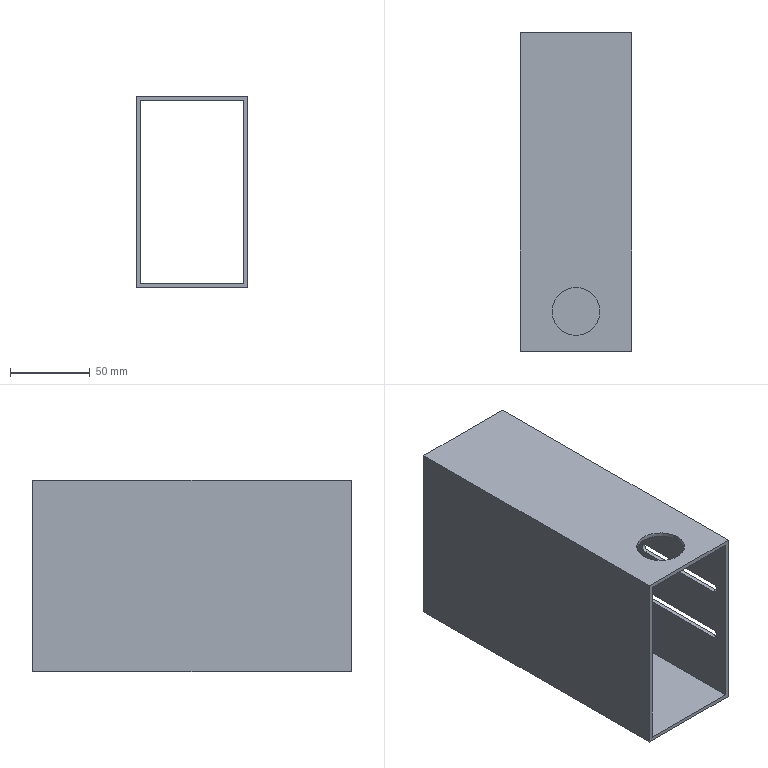Part | SolidWorks | features HoleWzd 2, Cut 1, Extrusion 1, ICE 1 | 1 solid | 34 faces | box 70 x 200 x 120 mm | volume 169957 mm3 | plane 22 | cylinder 12 | commonest cylinder face diameters 4.8 x6 5.8 x4 30 x2
STEP:
#1=CARTESIAN_POINT('',(67.5,52.4,-68.5));
#2=VERTEX_POINT('',#1);
#3=CARTESIAN_POINT('',(67.5,50.,-70.9));
#4=VERTEX_POINT('',#3);
#5=CARTESIAN_POINT('',(67.5,50.,-68.5));
#6=DIRECTION('',(-1.,0.,0.));
#7=DIRECTION('',(0.,0.,1.));
#8=AXIS2_PLACEMENT_3D('',#5,#6,#7);
#9=CIRCLE('',#8,2.4);
#10=EDGE_CURVE('',#2,#4,#9,.T.);
#11=ORIENTED_EDGE('',*,*,#10,.T.);
#12=CARTESIAN_POINT('',(70.,50.,-70.9));
#13=VERTEX_POINT('',#12);
#14=CARTESIAN_POINT('',(70.,50.,-70.9));
#15=DIRECTION('',(1.,0.,0.));
#16=VECTOR('',#15,1000.);
#17=LINE('',#14,#16);
#18=EDGE_CURVE('',#4,#13,#17,.T.);
#19=ORIENTED_EDGE('',*,*,#18,.T.);
#20=CARTESIAN_POINT('',(70.,52.4,-68.5));
#21=VERTEX_POINT('',#20);
#22=CARTESIAN_POINT('',(70.,50.,-68.5));
#23=DIRECTION('',(1.,0.,0.));
#24=DIRECTION('',(0.,0.,-1.));
#25=AXIS2_PLACEMENT_3D('',#22,#23,#24);
#26=CIRCLE('',#25,2.4);
#27=EDGE_CURVE('',#13,#21,#26,.T.);
#28=ORIENTED_EDGE('',*,*,#27,.T.);
#29=CARTESIAN_POINT('',(67.499,52.4,-68.5));
#30=DIRECTION('',(-1.,0.,0.));
#31=VECTOR('',#30,1000.);
#32=LINE('',#29,#31);
#33=EDGE_CURVE('',#21,#2,#32,.T.);
#34=ORIENTED_EDGE('',*,*,#33,.T.);
#35=EDGE_LOOP('',(#11,#19,#28,#34));
#36=FACE_OUTER_BOUND('',#35,.T.);
#37=CARTESIAN_POINT('',(70.,50.,-68.5));
#38=DIRECTION('',(1.,0.,0.));
#39=DIRECTION('',(0.,0.,-1.));
#40=AXIS2_PLACEMENT_3D('',#37,#38,#39);
#41=CYLINDRICAL_SURFACE('',#40,2.4);
#42=ADVANCED_FACE('',(#36),#41,.F.);
#43=CARTESIAN_POINT('',(67.5,22.4,-68.5));
#44=VERTEX_POINT('',#43);
#45=CARTESIAN_POINT('',(67.5,20.,-70.9));
#46=VERTEX_POINT('',#45);
#47=CARTESIAN_POINT('',(67.5,20.,-68.5));
#48=DIRECTION('',(-1.,0.,0.));
#49=DIRECTION('',(0.,0.,1.));
#50=AXIS2_PLACEMENT_3D('',#47,#48,#49);
#51=CIRCLE('',#50,2.4);
#52=EDGE_CURVE('',#44,#46,#51,.T.);
#53=ORIENTED_EDGE('',*,*,#52,.T.);
#54=CARTESIAN_POINT('',(70.,20.,-70.9));
#55=VERTEX_POINT('',#54);
#56=CARTESIAN_POINT('',(70.,20.,-70.9));
#57=DIRECTION('',(1.,0.,0.));
#58=VECTOR('',#57,1000.);
#59=LINE('',#56,#58);
#60=EDGE_CURVE('',#46,#55,#59,.T.);
#61=ORIENTED_EDGE('',*,*,#60,.T.);
#62=CARTESIAN_POINT('',(70.,22.4,-68.5));
#63=VERTEX_POINT('',#62);
#64=CARTESIAN_POINT('',(70.,20.,-68.5));
#65=DIRECTION('',(1.,0.,0.));
#66=DIRECTION('',(0.,0.,-1.));
#67=AXIS2_PLACEMENT_3D('',#64,#65,#66);
#68=CIRCLE('',#67,2.4);
#69=EDGE_CURVE('',#55,#63,#68,.T.);
#70=ORIENTED_EDGE('',*,*,#69,.T.);
#71=CARTESIAN_POINT('',(67.499,22.4,-68.5));
#72=DIRECTION('',(-1.,0.,0.));
#73=VECTOR('',#72,1000.);
#74=LINE('',#71,#73);
#75=EDGE_CURVE('',#63,#44,#74,.T.);
#76=ORIENTED_EDGE('',*,*,#75,.T.);
#77=EDGE_LOOP('',(#53,#61,#70,#76));
#78=FACE_OUTER_BOUND('',#77,.T.);
#79=CARTESIAN_POINT('',(70.,20.,-68.5));
#80=DIRECTION('',(1.,0.,0.));
#81=DIRECTION('',(0.,0.,-1.));
#82=AXIS2_PLACEMENT_3D('',#79,#80,#81);
#83=CYLINDRICAL_SURFACE('',#82,2.4);
#84=ADVANCED_FACE('',(#78),#83,.F.);
#85=CARTESIAN_POINT('',(20.,-75.,-2.5));
#86=VERTEX_POINT('',#85);
#87=CARTESIAN_POINT('',(50.,-75.,-2.5));
#88=VERTEX_POINT('',#87);
#89=CARTESIAN_POINT('',(35.,-75.,-2.5));
#90=DIRECTION('',(0.,0.,1.));
#91=DIRECTION('',(-1.,0.,0.));
#92=AXIS2_PLACEMENT_3D('',#89,#90,#91);
#93=CIRCLE('',#92,15.);
#94=EDGE_CURVE('',#86,#88,#93,.T.);
#95=ORIENTED_EDGE('',*,*,#94,.F.);
#96=CARTESIAN_POINT('',(20.,-75.,0.));
#97=VERTEX_POINT('',#96);
#98=CARTESIAN_POINT('',(20.,-75.,-120.001));
#99=DIRECTION('',(0.,0.,1.));
#100=VECTOR('',#99,1000.);
#101=LINE('',#98,#100);
#102=EDGE_CURVE('',#86,#97,#101,.T.);
#103=ORIENTED_EDGE('',*,*,#102,.T.);
#104=CARTESIAN_POINT('',(50.,-75.,0.));
#105=VERTEX_POINT('',#104);
#106=CARTESIAN_POINT('',(35.,-75.,0.));
#107=DIRECTION('',(0.,0.,1.));
#108=DIRECTION('',(1.,0.,0.));
#109=AXIS2_PLACEMENT_3D('',#106,#107,#108);
#110=CIRCLE('',#109,15.);
#111=EDGE_CURVE('',#97,#105,#110,.T.);
#112=ORIENTED_EDGE('',*,*,#111,.T.);
#113=CARTESIAN_POINT('',(50.,-75.,-120.001));
#114=DIRECTION('',(0.,0.,1.));
#115=VECTOR('',#114,1000.);
#116=LINE('',#113,#115);
#117=EDGE_CURVE('',#88,#105,#116,.T.);
#118=ORIENTED_EDGE('',*,*,#117,.F.);
#119=EDGE_LOOP('',(#95,#103,#112,#118));
#120=FACE_OUTER_BOUND('',#119,.T.);
#121=CARTESIAN_POINT('',(35.,-75.,-120.001));
#122=DIRECTION('',(0.,0.,1.));
#123=DIRECTION('',(1.,0.,0.));
#124=AXIS2_PLACEMENT_3D('',#121,#122,#123);
#125=CYLINDRICAL_SURFACE('',#124,15.);
#126=ADVANCED_FACE('',(#120),#125,.F.);
#127=CARTESIAN_POINT('',(70.,-89.,-43.452));
#128=VERTEX_POINT('',#127);
#129=CARTESIAN_POINT('',(70.,-29.,-43.452));
#130=VERTEX_POINT('',#129);
#131=CARTESIAN_POINT('',(70.,-89.,-43.452));
#132=DIRECTION('',(0.,1.,0.));
#133=VECTOR('',#132,1000.);
#134=LINE('',#131,#133);
#135=EDGE_CURVE('',#128,#130,#134,.T.);
#136=ORIENTED_EDGE('',*,*,#135,.F.);
#137=CARTESIAN_POINT('',(70.,-89.,-37.652));
#138=VERTEX_POINT('',#137);
#139=CARTESIAN_POINT('',(70.,-89.,-40.552));
#140=DIRECTION('',(1.,0.,0.));
#141=DIRECTION('',(0.,0.,-1.));
#142=AXIS2_PLACEMENT_3D('',#139,#140,#141);
#143=CIRCLE('',#142,2.9);
#144=EDGE_CURVE('',#138,#128,#143,.T.);
#145=ORIENTED_EDGE('',*,*,#144,.F.);
#146=CARTESIAN_POINT('',(70.,-29.,-37.652));
#147=VERTEX_POINT('',#146);
#148=CARTESIAN_POINT('',(70.,-89.,-37.652));
#149=DIRECTION('',(0.,1.,0.));
#150=VECTOR('',#149,1000.);
#151=LINE('',#148,#150);
#152=EDGE_CURVE('',#138,#147,#151,.T.);
#153=ORIENTED_EDGE('',*,*,#152,.T.);
#154=CARTESIAN_POINT('',(70.,-29.,-40.552));
#155=DIRECTION('',(1.,0.,0.));
#156=DIRECTION('',(0.,0.,-1.));
#157=AXIS2_PLACEMENT_3D('',#154,#155,#156);
#158=CIRCLE('',#157,2.9);
#159=EDGE_CURVE('',#130,#147,#158,.T.);
#160=ORIENTED_EDGE('',*,*,#159,.F.);
#161=EDGE_LOOP('',(#136,#145,#153,#160));
#162=FACE_BOUND('',#161,.T.);
#163=CARTESIAN_POINT('',(70.,22.4,-56.5));
#164=VERTEX_POINT('',#163);
#165=CARTESIAN_POINT('',(70.,17.6,-56.5));
#166=VERTEX_POINT('',#165);
#167=CARTESIAN_POINT('',(70.,20.,-56.5));
#168=DIRECTION('',(1.,0.,0.));
#169=DIRECTION('',(0.,0.,-1.));
#170=AXIS2_PLACEMENT_3D('',#167,#168,#169);
#171=CIRCLE('',#170,2.4);
#172=EDGE_CURVE('',#164,#166,#171,.T.);
#173=ORIENTED_EDGE('',*,*,#172,.F.);
#174=CARTESIAN_POINT('',(70.,22.4,-68.5));
#175=DIRECTION('',(0.,0.,1.));
#176=VECTOR('',#175,1000.);
#177=LINE('',#174,#176);
#178=EDGE_CURVE('',#63,#164,#177,.T.);
#179=ORIENTED_EDGE('',*,*,#178,.F.);
#180=ORIENTED_EDGE('',*,*,#69,.F.);
#181=CARTESIAN_POINT('',(70.,17.6,-68.5));
#182=VERTEX_POINT('',#181);
#183=CARTESIAN_POINT('',(70.,20.,-68.5));
#184=DIRECTION('',(1.,0.,0.));
#185=DIRECTION('',(0.,0.,-1.));
#186=AXIS2_PLACEMENT_3D('',#183,#184,#185);
#187=CIRCLE('',#186,2.4);
#188=EDGE_CURVE('',#182,#55,#187,.T.);
#189=ORIENTED_EDGE('',*,*,#188,.F.);
#190=CARTESIAN_POINT('',(70.,17.6,-68.5));
#191=DIRECTION('',(0.,0.,1.));
#192=VECTOR('',#191,1000.);
#193=LINE('',#190,#192);
#194=EDGE_CURVE('',#182,#166,#193,.T.);
#195=ORIENTED_EDGE('',*,*,#194,.T.);
#196=EDGE_LOOP('',(#173,#179,#180,#189,#195));
#197=FACE_BOUND('',#196,.T.);
#198=CARTESIAN_POINT('',(70.,-100.,0.));
#199=VERTEX_POINT('',#198);
#200=CARTESIAN_POINT('',(70.,-100.,-120.));
#201=VERTEX_POINT('',#200);
#202=CARTESIAN_POINT('',(70.,-100.,0.));
#203=DIRECTION('',(0.,0.,-1.));
#204=VECTOR('',#203,1000.);
#205=LINE('',#202,#204);
#206=EDGE_CURVE('',#199,#201,#205,.T.);
#207=ORIENTED_EDGE('',*,*,#206,.T.);
#208=CARTESIAN_POINT('',(70.,100.,-120.));
#209=VERTEX_POINT('',#208);
#210=CARTESIAN_POINT('',(70.,100.,-120.));
#211=DIRECTION('',(0.,-1.,0.));
#212=VECTOR('',#211,1000.);
#213=LINE('',#210,#212);
#214=EDGE_CURVE('',#209,#201,#213,.T.);
#215=ORIENTED_EDGE('',*,*,#214,.F.);
#216=CARTESIAN_POINT('',(70.,100.,0.));
#217=VERTEX_POINT('',#216);
#218=CARTESIAN_POINT('',(70.,100.,0.));
#219=DIRECTION('',(0.,0.,-1.));
#220=VECTOR('',#219,1000.);
#221=LINE('',#218,#220);
#222=EDGE_CURVE('',#217,#209,#221,.T.);
#223=ORIENTED_EDGE('',*,*,#222,.F.);
#224=CARTESIAN_POINT('',(70.,100.,0.));
#225=DIRECTION('',(0.,-1.,0.));
#226=VECTOR('',#225,1000.);
#227=LINE('',#224,#226);
#228=EDGE_CURVE('',#217,#199,#227,.T.);
#229=ORIENTED_EDGE('',*,*,#228,.T.);
#230=EDGE_LOOP('',(#207,#215,#223,#229));
#231=FACE_OUTER_BOUND('',#230,.T.);
#232=CARTESIAN_POINT('',(70.,52.4,-56.5));
#233=VERTEX_POINT('',#232);
#234=CARTESIAN_POINT('',(70.,52.4,-68.5));
#235=DIRECTION('',(0.,0.,1.));
#236=VECTOR('',#235,1000.);
#237=LINE('',#234,#236);
#238=EDGE_CURVE('',#21,#233,#237,.T.);
#239=ORIENTED_EDGE('',*,*,#238,.F.);
#240=ORIENTED_EDGE('',*,*,#27,.F.);
#241=CARTESIAN_POINT('',(70.,47.6,-68.5));
#242=VERTEX_POINT('',#241);
#243=CARTESIAN_POINT('',(70.,50.,-68.5));
#244=DIRECTION('',(1.,0.,0.));
#245=DIRECTION('',(0.,0.,-1.));
#246=AXIS2_PLACEMENT_3D('',#243,#244,#245);
#247=CIRCLE('',#246,2.4);
#248=EDGE_CURVE('',#242,#13,#247,.T.);
#249=ORIENTED_EDGE('',*,*,#248,.F.);
#250=CARTESIAN_POINT('',(70.,47.6,-56.5));
#251=VERTEX_POINT('',#250);
#252=CARTESIAN_POINT('',(70.,47.6,-68.5));
#253=DIRECTION('',(0.,0.,1.));
#254=VECTOR('',#253,1000.);
#255=LINE('',#252,#254);
#256=EDGE_CURVE('',#242,#251,#255,.T.);
#257=ORIENTED_EDGE('',*,*,#256,.T.);
#258=CARTESIAN_POINT('',(70.,50.,-56.5));
#259=DIRECTION('',(1.,0.,0.));
#260=DIRECTION('',(0.,0.,-1.));
#261=AXIS2_PLACEMENT_3D('',#258,#259,#260);
#262=CIRCLE('',#261,2.4);
#263=EDGE_CURVE('',#233,#251,#262,.T.);
#264=ORIENTED_EDGE('',*,*,#263,.F.);
#265=EDGE_LOOP('',(#239,#240,#249,#257,#264));
#266=FACE_BOUND('',#265,.T.);
#267=CARTESIAN_POINT('',(70.,-89.,-78.452));
#268=VERTEX_POINT('',#267);
#269=CARTESIAN_POINT('',(70.,-29.,-78.452));
#270=VERTEX_POINT('',#269);
#271=CARTESIAN_POINT('',(70.,-89.,-78.452));
#272=DIRECTION('',(0.,1.,0.));
#273=VECTOR('',#272,1000.);
#274=LINE('',#271,#273);
#275=EDGE_CURVE('',#268,#270,#274,.T.);
#276=ORIENTED_EDGE('',*,*,#275,.F.);
#277=CARTESIAN_POINT('',(70.,-89.,-72.652));
#278=VERTEX_POINT('',#277);
#279=CARTESIAN_POINT('',(70.,-89.,-75.552));
#280=DIRECTION('',(1.,0.,0.));
#281=DIRECTION('',(0.,0.,-1.));
#282=AXIS2_PLACEMENT_3D('',#279,#280,#281);
#283=CIRCLE('',#282,2.9);
#284=EDGE_CURVE('',#278,#268,#283,.T.);
#285=ORIENTED_EDGE('',*,*,#284,.F.);
#286=CARTESIAN_POINT('',(70.,-29.,-72.652));
#287=VERTEX_POINT('',#286);
#288=CARTESIAN_POINT('',(70.,-89.,-72.652));
#289=DIRECTION('',(0.,1.,0.));
#290=VECTOR('',#289,1000.);
#291=LINE('',#288,#290);
#292=EDGE_CURVE('',#278,#287,#291,.T.);
#293=ORIENTED_EDGE('',*,*,#292,.T.);
#294=CARTESIAN_POINT('',(70.,-29.,-75.552));
#295=DIRECTION('',(1.,0.,0.));
#296=DIRECTION('',(0.,0.,-1.));
#297=AXIS2_PLACEMENT_3D('',#294,#295,#296);
#298=CIRCLE('',#297,2.9);
#299=EDGE_CURVE('',#270,#287,#298,.T.);
#300=ORIENTED_EDGE('',*,*,#299,.F.);
#301=EDGE_LOOP('',(#276,#285,#293,#300));
#302=FACE_BOUND('',#301,.T.);
#303=CARTESIAN_POINT('',(70.,100.,0.));
#304=DIRECTION('',(-1.,0.,0.));
#305=DIRECTION('',(0.,0.,1.));
#306=AXIS2_PLACEMENT_3D('',#303,#304,#305);
#307=PLANE('',#306);
#308=ADVANCED_FACE('',(#162,#197,#231,#266,#302),#307,.F.);
#309=CARTESIAN_POINT('',(0.,100.,-120.));
#310=VERTEX_POINT('',#309);
#311=CARTESIAN_POINT('',(0.,100.,0.));
#312=VERTEX_POINT('',#311);
#313=CARTESIAN_POINT('',(0.,100.,0.));
#314=DIRECTION('',(0.,0.,1.));
#315=VECTOR('',#314,1000.);
#316=LINE('',#313,#315);
#317=EDGE_CURVE('',#310,#312,#316,.T.);
#318=ORIENTED_EDGE('',*,*,#317,.T.);
#319=CARTESIAN_POINT('',(0.,100.,0.));
#320=DIRECTION('',(1.,0.,0.));
#321=VECTOR('',#320,1000.);
#322=LINE('',#319,#321);
#323=EDGE_CURVE('',#312,#217,#322,.T.);
#324=ORIENTED_EDGE('',*,*,#323,.T.);
#325=ORIENTED_EDGE('',*,*,#222,.T.);
#326=CARTESIAN_POINT('',(0.,100.,-120.));
#327=DIRECTION('',(-1.,0.,0.));
#328=VECTOR('',#327,1000.);
#329=LINE('',#326,#328);
#330=EDGE_CURVE('',#209,#310,#329,.T.);
#331=ORIENTED_EDGE('',*,*,#330,.T.);
#332=EDGE_LOOP('',(#318,#324,#325,#331));
#333=FACE_OUTER_BOUND('',#332,.T.);
#334=CARTESIAN_POINT('',(2.5,100.,-117.5));
#335=VERTEX_POINT('',#334);
#336=CARTESIAN_POINT('',(2.5,100.,-2.5));
#337=VERTEX_POINT('',#336);
#338=CARTESIAN_POINT('',(2.5,100.,-2.5));
#339=DIRECTION('',(0.,0.,1.));
#340=VECTOR('',#339,1000.);
#341=LINE('',#338,#340);
#342=EDGE_CURVE('',#335,#337,#341,.T.);
#343=ORIENTED_EDGE('',*,*,#342,.F.);
#344=CARTESIAN_POINT('',(67.5,100.,-117.5));
#345=VERTEX_POINT('',#344);
#346=CARTESIAN_POINT('',(2.5,100.,-117.5));
#347=DIRECTION('',(-1.,0.,0.));
#348=VECTOR('',#347,1000.);
#349=LINE('',#346,#348);
#350=EDGE_CURVE('',#345,#335,#349,.T.);
#351=ORIENTED_EDGE('',*,*,#350,.F.);
#352=CARTESIAN_POINT('',(67.5,100.,-2.5));
#353=VERTEX_POINT('',#352);
#354=CARTESIAN_POINT('',(67.5,100.,-2.5));
#355=DIRECTION('',(0.,0.,-1.));
#356=VECTOR('',#355,1000.);
#357=LINE('',#354,#356);
#358=EDGE_CURVE('',#353,#345,#357,.T.);
#359=ORIENTED_EDGE('',*,*,#358,.F.);
#360=CARTESIAN_POINT('',(2.5,100.,-2.5));
#361=DIRECTION('',(1.,0.,0.));
#362=VECTOR('',#361,1000.);
#363=LINE('',#360,#362);
#364=EDGE_CURVE('',#337,#353,#363,.T.);
#365=ORIENTED_EDGE('',*,*,#364,.F.);
#366=EDGE_LOOP('',(#343,#351,#359,#365));
#367=FACE_BOUND('',#366,.T.);
#368=CARTESIAN_POINT('',(0.,100.,0.));
#369=DIRECTION('',(0.,-1.,0.));
#370=DIRECTION('',(0.,0.,-1.));
#371=AXIS2_PLACEMENT_3D('',#368,#369,#370);
#372=PLANE('',#371);
#373=ADVANCED_FACE('',(#333,#367),#372,.F.);
#374=CARTESIAN_POINT('',(0.,-100.,-120.));
#375=VERTEX_POINT('',#374);
#376=CARTESIAN_POINT('',(0.,-100.,0.));
#377=VERTEX_POINT('',#376);
#378=CARTESIAN_POINT('',(0.,-100.,0.));
#379=DIRECTION('',(0.,0.,1.));
#380=VECTOR('',#379,1000.);
#381=LINE('',#378,#380);
#382=EDGE_CURVE('',#375,#377,#381,.T.);
#383=ORIENTED_EDGE('',*,*,#382,.F.);
#384=CARTESIAN_POINT('',(0.,-100.,-120.));
#385=DIRECTION('',(-1.,0.,0.));
#386=VECTOR('',#385,1000.);
#387=LINE('',#384,#386);
#388=EDGE_CURVE('',#201,#375,#387,.T.);
#389=ORIENTED_EDGE('',*,*,#388,.F.);
#390=ORIENTED_EDGE('',*,*,#206,.F.);
#391=CARTESIAN_POINT('',(0.,-100.,0.));
#392=DIRECTION('',(1.,0.,0.));
#393=VECTOR('',#392,1000.);
#394=LINE('',#391,#393);
#395=EDGE_CURVE('',#377,#199,#394,.T.);
#396=ORIENTED_EDGE('',*,*,#395,.F.);
#397=EDGE_LOOP('',(#383,#389,#390,#396));
#398=FACE_OUTER_BOUND('',#397,.T.);
#399=CARTESIAN_POINT('',(67.5,-100.,-117.5));
#400=VERTEX_POINT('',#399);
#401=CARTESIAN_POINT('',(2.5,-100.,-117.5));
#402=VERTEX_POINT('',#401);
#403=CARTESIAN_POINT('',(2.5,-100.,-117.5));
#404=DIRECTION('',(-1.,0.,0.));
#405=VECTOR('',#404,1000.);
#406=LINE('',#403,#405);
#407=EDGE_CURVE('',#400,#402,#406,.T.);
#408=ORIENTED_EDGE('',*,*,#407,.T.);
#409=CARTESIAN_POINT('',(2.5,-100.,-2.5));
#410=VERTEX_POINT('',#409);
#411=CARTESIAN_POINT('',(2.5,-100.,-2.5));
#412=DIRECTION('',(0.,0.,1.));
#413=VECTOR('',#412,1000.);
#414=LINE('',#411,#413);
#415=EDGE_CURVE('',#402,#410,#414,.T.);
#416=ORIENTED_EDGE('',*,*,#415,.T.);
#417=CARTESIAN_POINT('',(67.5,-100.,-2.5));
#418=VERTEX_POINT('',#417);
#419=CARTESIAN_POINT('',(2.5,-100.,-2.5));
#420=DIRECTION('',(1.,0.,0.));
#421=VECTOR('',#420,1000.);
#422=LINE('',#419,#421);
#423=EDGE_CURVE('',#410,#418,#422,.T.);
#424=ORIENTED_EDGE('',*,*,#423,.T.);
#425=CARTESIAN_POINT('',(67.5,-100.,-2.5));
#426=DIRECTION('',(0.,0.,-1.));
#427=VECTOR('',#426,1000.);
#428=LINE('',#425,#427);
#429=EDGE_CURVE('',#418,#400,#428,.T.);
#430=ORIENTED_EDGE('',*,*,#429,.T.);
#431=EDGE_LOOP('',(#408,#416,#424,#430));
#432=FACE_BOUND('',#431,.T.);
#433=CARTESIAN_POINT('',(0.,-100.,0.));
#434=DIRECTION('',(0.,-1.,0.));
#435=DIRECTION('',(0.,0.,-1.));
#436=AXIS2_PLACEMENT_3D('',#433,#434,#435);
#437=PLANE('',#436);
#438=ADVANCED_FACE('',(#398,#432),#437,.T.);
#439=ORIENTED_EDGE('',*,*,#382,.T.);
#440=CARTESIAN_POINT('',(0.,100.,0.));
#441=DIRECTION('',(0.,-1.,0.));
#442=VECTOR('',#441,1000.);
#443=LINE('',#440,#442);
#444=EDGE_CURVE('',#312,#377,#443,.T.);
#445=ORIENTED_EDGE('',*,*,#444,.F.);
#446=ORIENTED_EDGE('',*,*,#317,.F.);
#447=CARTESIAN_POINT('',(0.,100.,-120.));
#448=DIRECTION('',(0.,-1.,0.));
#449=VECTOR('',#448,1000.);
#450=LINE('',#447,#449);
#451=EDGE_CURVE('',#310,#375,#450,.T.);
#452=ORIENTED_EDGE('',*,*,#451,.T.);
#453=EDGE_LOOP('',(#439,#445,#446,#452));
#454=FACE_OUTER_BOUND('',#453,.T.);
#455=CARTESIAN_POINT('',(0.,100.,0.));
#456=DIRECTION('',(1.,0.,0.));
#457=DIRECTION('',(0.,0.,-1.));
#458=AXIS2_PLACEMENT_3D('',#455,#456,#457);
#459=PLANE('',#458);
#460=ADVANCED_FACE('',(#454),#459,.F.);
#461=CARTESIAN_POINT('',(35.,-75.,0.));
#462=DIRECTION('',(0.,0.,1.));
#463=DIRECTION('',(1.,0.,0.));
#464=AXIS2_PLACEMENT_3D('',#461,#462,#463);
#465=CIRCLE('',#464,15.);
#466=EDGE_CURVE('',#105,#97,#465,.T.);
#467=ORIENTED_EDGE('',*,*,#466,.F.);
#468=ORIENTED_EDGE('',*,*,#111,.F.);
#469=EDGE_LOOP('',(#467,#468));
#470=FACE_BOUND('',#469,.T.);
#471=ORIENTED_EDGE('',*,*,#395,.T.);
#472=ORIENTED_EDGE('',*,*,#228,.F.);
#473=ORIENTED_EDGE('',*,*,#323,.F.);
#474=ORIENTED_EDGE('',*,*,#444,.T.);
#475=EDGE_LOOP('',(#471,#472,#473,#474));
#476=FACE_OUTER_BOUND('',#475,.T.);
#477=CARTESIAN_POINT('',(0.,100.,0.));
#478=DIRECTION('',(0.,0.,-1.));
#479=DIRECTION('',(-1.,0.,0.));
#480=AXIS2_PLACEMENT_3D('',#477,#478,#479);
#481=PLANE('',#480);
#482=ADVANCED_FACE('',(#470,#476),#481,.F.);
#483=CARTESIAN_POINT('',(53.,74.,-120.));
#484=VERTEX_POINT('',#483);
#485=CARTESIAN_POINT('',(53.,-24.,-120.));
#486=VERTEX_POINT('',#485);
#487=CARTESIAN_POINT('',(53.,-24.,-120.));
#488=DIRECTION('',(0.,-1.,0.));
#489=VECTOR('',#488,1000.);
#490=LINE('',#487,#489);
#491=EDGE_CURVE('',#484,#486,#490,.T.);
#492=ORIENTED_EDGE('',*,*,#491,.F.);
#493=CARTESIAN_POINT('',(8.,74.,-120.));
#494=VERTEX_POINT('',#493);
#495=CARTESIAN_POINT('',(53.,74.,-120.));
#496=DIRECTION('',(1.,0.,0.));
#497=VECTOR('',#496,1000.);
#498=LINE('',#495,#497);
#499=EDGE_CURVE('',#494,#484,#498,.T.);
#500=ORIENTED_EDGE('',*,*,#499,.F.);
#501=CARTESIAN_POINT('',(8.,-24.,-120.));
#502=VERTEX_POINT('',#501);
#503=CARTESIAN_POINT('',(8.,-24.,-120.));
#504=DIRECTION('',(0.,1.,0.));
#505=VECTOR('',#504,1000.);
#506=LINE('',#503,#505);
#507=EDGE_CURVE('',#502,#494,#506,.T.);
#508=ORIENTED_EDGE('',*,*,#507,.F.);
#509=CARTESIAN_POINT('',(53.,-24.,-120.));
#510=DIRECTION('',(-1.,0.,0.));
#511=VECTOR('',#510,1000.);
#512=LINE('',#509,#511);
#513=EDGE_CURVE('',#486,#502,#512,.T.);
#514=ORIENTED_EDGE('',*,*,#513,.F.);
#515=EDGE_LOOP('',(#492,#500,#508,#514));
#516=FACE_BOUND('',#515,.T.);
#517=ORIENTED_EDGE('',*,*,#388,.T.);
#518=ORIENTED_EDGE('',*,*,#451,.F.);
#519=ORIENTED_EDGE('',*,*,#330,.F.);
#520=ORIENTED_EDGE('',*,*,#214,.T.);
#521=EDGE_LOOP('',(#517,#518,#519,#520));
#522=FACE_OUTER_BOUND('',#521,.T.);
#523=CARTESIAN_POINT('',(0.,100.,-120.));
#524=DIRECTION('',(0.,0.,1.));
#525=DIRECTION('',(1.,0.,0.));
#526=AXIS2_PLACEMENT_3D('',#523,#524,#525);
#527=PLANE('',#526);
#528=ADVANCED_FACE('',(#516,#522),#527,.F.);
#529=ORIENTED_EDGE('',*,*,#415,.F.);
#530=CARTESIAN_POINT('',(2.5,100.,-117.5));
#531=DIRECTION('',(0.,-1.,0.));
#532=VECTOR('',#531,1000.);
#533=LINE('',#530,#532);
#534=EDGE_CURVE('',#335,#402,#533,.T.);
#535=ORIENTED_EDGE('',*,*,#534,.F.);
#536=ORIENTED_EDGE('',*,*,#342,.T.);
#537=CARTESIAN_POINT('',(2.5,100.,-2.5));
#538=DIRECTION('',(0.,-1.,0.));
#539=VECTOR('',#538,1000.);
#540=LINE('',#537,#539);
#541=EDGE_CURVE('',#337,#410,#540,.T.);
#542=ORIENTED_EDGE('',*,*,#541,.T.);
#543=EDGE_LOOP('',(#529,#535,#536,#542));
#544=FACE_OUTER_BOUND('',#543,.T.);
#545=CARTESIAN_POINT('',(2.5,100.,-2.5));
#546=DIRECTION('',(1.,0.,0.));
#547=DIRECTION('',(0.,0.,-1.));
#548=AXIS2_PLACEMENT_3D('',#545,#546,#547);
#549=PLANE('',#548);
#550=ADVANCED_FACE('',(#544),#549,.T.);
#551=CARTESIAN_POINT('',(35.,-75.,-2.5));
#552=DIRECTION('',(0.,0.,1.));
#553=DIRECTION('',(-1.,0.,0.));
#554=AXIS2_PLACEMENT_3D('',#551,#552,#553);
#555=CIRCLE('',#554,15.);
#556=EDGE_CURVE('',#88,#86,#555,.T.);
#557=ORIENTED_EDGE('',*,*,#556,.T.);
#558=ORIENTED_EDGE('',*,*,#94,.T.);
#559=EDGE_LOOP('',(#557,#558));
#560=FACE_BOUND('',#559,.T.);
#561=ORIENTED_EDGE('',*,*,#423,.F.);
#562=ORIENTED_EDGE('',*,*,#541,.F.);
#563=ORIENTED_EDGE('',*,*,#364,.T.);
#564=CARTESIAN_POINT('',(67.5,100.,-2.5));
#565=DIRECTION('',(0.,-1.,0.));
#566=VECTOR('',#565,1000.);
#567=LINE('',#564,#566);
#568=EDGE_CURVE('',#353,#418,#567,.T.);
#569=ORIENTED_EDGE('',*,*,#568,.T.);
#570=EDGE_LOOP('',(#561,#562,#563,#569));
#571=FACE_OUTER_BOUND('',#570,.T.);
#572=CARTESIAN_POINT('',(2.5,100.,-2.5));
#573=DIRECTION('',(0.,0.,-1.));
#574=DIRECTION('',(-1.,0.,0.));
#575=AXIS2_PLACEMENT_3D('',#572,#573,#574);
#576=PLANE('',#575);
#577=ADVANCED_FACE('',(#560,#571),#576,.T.);
#578=CARTESIAN_POINT('',(67.5,-89.,-72.652));
#579=VERTEX_POINT('',#578);
#580=CARTESIAN_POINT('',(67.5,-29.,-72.652));
#581=VERTEX_POINT('',#580);
#582=CARTESIAN_POINT('',(67.5,100.,-72.652));
#583=DIRECTION('',(0.,1.,0.));
#584=VECTOR('',#583,1000.);
#585=LINE('',#582,#584);
#586=EDGE_CURVE('',#579,#581,#585,.T.);
#587=ORIENTED_EDGE('',*,*,#586,.F.);
#588=CARTESIAN_POINT('',(67.5,-89.,-78.452));
#589=VERTEX_POINT('',#588);
#590=CARTESIAN_POINT('',(67.5,-89.,-75.552));
#591=DIRECTION('',(-1.,0.,0.));
#592=DIRECTION('',(0.,0.,1.));
#593=AXIS2_PLACEMENT_3D('',#590,#591,#592);
#594=CIRCLE('',#593,2.9);
#595=EDGE_CURVE('',#589,#579,#594,.T.);
#596=ORIENTED_EDGE('',*,*,#595,.F.);
#597=CARTESIAN_POINT('',(67.5,-29.,-78.452));
#598=VERTEX_POINT('',#597);
#599=CARTESIAN_POINT('',(67.5,100.,-78.452));
#600=DIRECTION('',(0.,-1.,0.));
#601=VECTOR('',#600,1000.);
#602=LINE('',#599,#601);
#603=EDGE_CURVE('',#598,#589,#602,.T.);
#604=ORIENTED_EDGE('',*,*,#603,.F.);
#605=CARTESIAN_POINT('',(67.5,-29.,-75.552));
#606=DIRECTION('',(-1.,0.,0.));
#607=DIRECTION('',(0.,0.,1.));
#608=AXIS2_PLACEMENT_3D('',#605,#606,#607);
#609=CIRCLE('',#608,2.9);
#610=EDGE_CURVE('',#581,#598,#609,.T.);
#611=ORIENTED_EDGE('',*,*,#610,.F.);
#612=EDGE_LOOP('',(#587,#596,#604,#611));
#613=FACE_BOUND('',#612,.T.);
#614=CARTESIAN_POINT('',(67.5,-89.,-37.652));
#615=VERTEX_POINT('',#614);
#616=CARTESIAN_POINT('',(67.5,-29.,-37.652));
#617=VERTEX_POINT('',#616);
#618=CARTESIAN_POINT('',(67.5,100.,-37.652));
#619=DIRECTION('',(0.,1.,0.));
#620=VECTOR('',#619,1000.);
#621=LINE('',#618,#620);
#622=EDGE_CURVE('',#615,#617,#621,.T.);
#623=ORIENTED_EDGE('',*,*,#622,.F.);
#624=CARTESIAN_POINT('',(67.5,-89.,-43.452));
#625=VERTEX_POINT('',#624);
#626=CARTESIAN_POINT('',(67.5,-89.,-40.552));
#627=DIRECTION('',(-1.,0.,0.));
#628=DIRECTION('',(0.,0.,1.));
#629=AXIS2_PLACEMENT_3D('',#626,#627,#628);
#630=CIRCLE('',#629,2.9);
#631=EDGE_CURVE('',#625,#615,#630,.T.);
#632=ORIENTED_EDGE('',*,*,#631,.F.);
#633=CARTESIAN_POINT('',(67.5,-29.,-43.452));
#634=VERTEX_POINT('',#633);
#635=CARTESIAN_POINT('',(67.5,100.,-43.452));
#636=DIRECTION('',(0.,-1.,0.));
#637=VECTOR('',#636,1000.);
#638=LINE('',#635,#637);
#639=EDGE_CURVE('',#634,#625,#638,.T.);
#640=ORIENTED_EDGE('',*,*,#639,.F.);
#641=CARTESIAN_POINT('',(67.5,-29.,-40.552));
#642=DIRECTION('',(-1.,0.,0.));
#643=DIRECTION('',(0.,0.,1.));
#644=AXIS2_PLACEMENT_3D('',#641,#642,#643);
#645=CIRCLE('',#644,2.9);
#646=EDGE_CURVE('',#617,#634,#645,.T.);
#647=ORIENTED_EDGE('',*,*,#646,.F.);
#648=EDGE_LOOP('',(#623,#632,#640,#647));
#649=FACE_BOUND('',#648,.T.);
#650=CARTESIAN_POINT('',(67.5,47.6,-68.5));
#651=VERTEX_POINT('',#650);
#652=CARTESIAN_POINT('',(67.5,47.6,-56.5));
#653=VERTEX_POINT('',#652);
#654=CARTESIAN_POINT('',(67.5,47.6,-2.5));
#655=DIRECTION('',(0.,0.,1.));
#656=VECTOR('',#655,1000.);
#657=LINE('',#654,#656);
#658=EDGE_CURVE('',#651,#653,#657,.T.);
#659=ORIENTED_EDGE('',*,*,#658,.F.);
#660=CARTESIAN_POINT('',(67.5,50.,-68.5));
#661=DIRECTION('',(-1.,0.,0.));
#662=DIRECTION('',(0.,0.,1.));
#663=AXIS2_PLACEMENT_3D('',#660,#661,#662);
#664=CIRCLE('',#663,2.4);
#665=EDGE_CURVE('',#4,#651,#664,.T.);
#666=ORIENTED_EDGE('',*,*,#665,.F.);
#667=ORIENTED_EDGE('',*,*,#10,.F.);
#668=CARTESIAN_POINT('',(67.5,52.4,-56.5));
#669=VERTEX_POINT('',#668);
#670=CARTESIAN_POINT('',(67.5,52.4,-2.5));
#671=DIRECTION('',(0.,0.,-1.));
#672=VECTOR('',#671,1000.);
#673=LINE('',#670,#672);
#674=EDGE_CURVE('',#669,#2,#673,.T.);
#675=ORIENTED_EDGE('',*,*,#674,.F.);
#676=CARTESIAN_POINT('',(67.5,50.,-56.5));
#677=DIRECTION('',(-1.,0.,0.));
#678=DIRECTION('',(0.,0.,1.));
#679=AXIS2_PLACEMENT_3D('',#676,#677,#678);
#680=CIRCLE('',#679,2.4);
#681=EDGE_CURVE('',#653,#669,#680,.T.);
#682=ORIENTED_EDGE('',*,*,#681,.F.);
#683=EDGE_LOOP('',(#659,#666,#667,#675,#682));
#684=FACE_BOUND('',#683,.T.);
#685=CARTESIAN_POINT('',(67.5,17.6,-68.5));
#686=VERTEX_POINT('',#685);
#687=CARTESIAN_POINT('',(67.5,17.6,-56.5));
#688=VERTEX_POINT('',#687);
#689=CARTESIAN_POINT('',(67.5,17.6,-2.5));
#690=DIRECTION('',(0.,0.,1.));
#691=VECTOR('',#690,1000.);
#692=LINE('',#689,#691);
#693=EDGE_CURVE('',#686,#688,#692,.T.);
#694=ORIENTED_EDGE('',*,*,#693,.F.);
#695=CARTESIAN_POINT('',(67.5,20.,-68.5));
#696=DIRECTION('',(-1.,0.,0.));
#697=DIRECTION('',(0.,0.,1.));
#698=AXIS2_PLACEMENT_3D('',#695,#696,#697);
#699=CIRCLE('',#698,2.4);
#700=EDGE_CURVE('',#46,#686,#699,.T.);
#701=ORIENTED_EDGE('',*,*,#700,.F.);
#702=ORIENTED_EDGE('',*,*,#52,.F.);
#703=CARTESIAN_POINT('',(67.5,22.4,-56.5));
#704=VERTEX_POINT('',#703);
#705=CARTESIAN_POINT('',(67.5,22.4,-2.5));
#706=DIRECTION('',(0.,0.,-1.));
#707=VECTOR('',#706,1000.);
#708=LINE('',#705,#707);
#709=EDGE_CURVE('',#704,#44,#708,.T.);
#710=ORIENTED_EDGE('',*,*,#709,.F.);
#711=CARTESIAN_POINT('',(67.5,20.,-56.5));
#712=DIRECTION('',(-1.,0.,0.));
#713=DIRECTION('',(0.,0.,1.));
#714=AXIS2_PLACEMENT_3D('',#711,#712,#713);
#715=CIRCLE('',#714,2.4);
#716=EDGE_CURVE('',#688,#704,#715,.T.);
#717=ORIENTED_EDGE('',*,*,#716,.F.);
#718=EDGE_LOOP('',(#694,#701,#702,#710,#717));
#719=FACE_BOUND('',#718,.T.);
#720=ORIENTED_EDGE('',*,*,#429,.F.);
#721=ORIENTED_EDGE('',*,*,#568,.F.);
#722=ORIENTED_EDGE('',*,*,#358,.T.);
#723=CARTESIAN_POINT('',(67.5,100.,-117.5));
#724=DIRECTION('',(0.,-1.,0.));
#725=VECTOR('',#724,1000.);
#726=LINE('',#723,#725);
#727=EDGE_CURVE('',#345,#400,#726,.T.);
#728=ORIENTED_EDGE('',*,*,#727,.T.);
#729=EDGE_LOOP('',(#720,#721,#722,#728));
#730=FACE_OUTER_BOUND('',#729,.T.);
#731=CARTESIAN_POINT('',(67.5,100.,-2.5));
#732=DIRECTION('',(-1.,0.,0.));
#733=DIRECTION('',(0.,0.,1.));
#734=AXIS2_PLACEMENT_3D('',#731,#732,#733);
#735=PLANE('',#734);
#736=ADVANCED_FACE('',(#613,#649,#684,#719,#730),#735,.T.);
#737=CARTESIAN_POINT('',(8.,74.,-117.5));
#738=VERTEX_POINT('',#737);
#739=CARTESIAN_POINT('',(53.,74.,-117.5));
#740=VERTEX_POINT('',#739);
#741=CARTESIAN_POINT('',(53.,74.,-117.5));
#742=DIRECTION('',(1.,0.,0.));
#743=VECTOR('',#742,1000.);
#744=LINE('',#741,#743);
#745=EDGE_CURVE('',#738,#740,#744,.T.);
#746=ORIENTED_EDGE('',*,*,#745,.T.);
#747=CARTESIAN_POINT('',(53.,-24.,-117.5));
#748=VERTEX_POINT('',#747);
#749=CARTESIAN_POINT('',(53.,-24.,-117.5));
#750=DIRECTION('',(0.,-1.,0.));
#751=VECTOR('',#750,1000.);
#752=LINE('',#749,#751);
#753=EDGE_CURVE('',#740,#748,#752,.T.);
#754=ORIENTED_EDGE('',*,*,#753,.T.);
#755=CARTESIAN_POINT('',(8.,-24.,-117.5));
#756=VERTEX_POINT('',#755);
#757=CARTESIAN_POINT('',(53.,-24.,-117.5));
#758=DIRECTION('',(-1.,0.,0.));
#759=VECTOR('',#758,1000.);
#760=LINE('',#757,#759);
#761=EDGE_CURVE('',#748,#756,#760,.T.);
#762=ORIENTED_EDGE('',*,*,#761,.T.);
#763=CARTESIAN_POINT('',(8.,-24.,-117.5));
#764=DIRECTION('',(0.,1.,0.));
#765=VECTOR('',#764,1000.);
#766=LINE('',#763,#765);
#767=EDGE_CURVE('',#756,#738,#766,.T.);
#768=ORIENTED_EDGE('',*,*,#767,.T.);
#769=EDGE_LOOP('',(#746,#754,#762,#768));
#770=FACE_BOUND('',#769,.T.);
#771=ORIENTED_EDGE('',*,*,#407,.F.);
#772=ORIENTED_EDGE('',*,*,#727,.F.);
#773=ORIENTED_EDGE('',*,*,#350,.T.);
#774=ORIENTED_EDGE('',*,*,#534,.T.);
#775=EDGE_LOOP('',(#771,#772,#773,#774));
#776=FACE_OUTER_BOUND('',#775,.T.);
#777=CARTESIAN_POINT('',(2.5,100.,-117.5));
#778=DIRECTION('',(0.,0.,1.));
#779=DIRECTION('',(1.,0.,0.));
#780=AXIS2_PLACEMENT_3D('',#777,#778,#779);
#781=PLANE('',#780);
#782=ADVANCED_FACE('',(#770,#776),#781,.T.);
#783=CARTESIAN_POINT('',(8.,74.,0.001));
#784=DIRECTION('',(0.,0.,-1.));
#785=VECTOR('',#784,1000.);
#786=LINE('',#783,#785);
#787=EDGE_CURVE('',#738,#494,#786,.T.);
#788=ORIENTED_EDGE('',*,*,#787,.T.);
#789=ORIENTED_EDGE('',*,*,#499,.T.);
#790=CARTESIAN_POINT('',(53.,74.,0.001));
#791=DIRECTION('',(0.,0.,-1.));
#792=VECTOR('',#791,1000.);
#793=LINE('',#790,#792);
#794=EDGE_CURVE('',#740,#484,#793,.T.);
#795=ORIENTED_EDGE('',*,*,#794,.F.);
#796=ORIENTED_EDGE('',*,*,#745,.F.);
#797=EDGE_LOOP('',(#788,#789,#795,#796));
#798=FACE_OUTER_BOUND('',#797,.T.);
#799=CARTESIAN_POINT('',(53.,74.,0.001));
#800=DIRECTION('',(0.,1.,0.));
#801=DIRECTION('',(0.,0.,1.));
#802=AXIS2_PLACEMENT_3D('',#799,#800,#801);
#803=PLANE('',#802);
#804=ADVANCED_FACE('',(#798),#803,.F.);
#805=ORIENTED_EDGE('',*,*,#794,.T.);
#806=ORIENTED_EDGE('',*,*,#491,.T.);
#807=CARTESIAN_POINT('',(53.,-24.,0.001));
#808=DIRECTION('',(0.,0.,-1.));
#809=VECTOR('',#808,1000.);
#810=LINE('',#807,#809);
#811=EDGE_CURVE('',#748,#486,#810,.T.);
#812=ORIENTED_EDGE('',*,*,#811,.F.);
#813=ORIENTED_EDGE('',*,*,#753,.F.);
#814=EDGE_LOOP('',(#805,#806,#812,#813));
#815=FACE_OUTER_BOUND('',#814,.T.);
#816=CARTESIAN_POINT('',(53.,-24.,0.001));
#817=DIRECTION('',(1.,0.,0.));
#818=DIRECTION('',(0.,0.,-1.));
#819=AXIS2_PLACEMENT_3D('',#816,#817,#818);
#820=PLANE('',#819);
#821=ADVANCED_FACE('',(#815),#820,.F.);
#822=ORIENTED_EDGE('',*,*,#811,.T.);
#823=ORIENTED_EDGE('',*,*,#513,.T.);
#824=CARTESIAN_POINT('',(8.,-24.,0.001));
#825=DIRECTION('',(0.,0.,-1.));
#826=VECTOR('',#825,1000.);
#827=LINE('',#824,#826);
#828=EDGE_CURVE('',#756,#502,#827,.T.);
#829=ORIENTED_EDGE('',*,*,#828,.F.);
#830=ORIENTED_EDGE('',*,*,#761,.F.);
#831=EDGE_LOOP('',(#822,#823,#829,#830));
#832=FACE_OUTER_BOUND('',#831,.T.);
#833=CARTESIAN_POINT('',(53.,-24.,0.001));
#834=DIRECTION('',(0.,-1.,0.));
#835=DIRECTION('',(0.,0.,-1.));
#836=AXIS2_PLACEMENT_3D('',#833,#834,#835);
#837=PLANE('',#836);
#838=ADVANCED_FACE('',(#832),#837,.F.);
#839=ORIENTED_EDGE('',*,*,#828,.T.);
#840=ORIENTED_EDGE('',*,*,#507,.T.);
#841=ORIENTED_EDGE('',*,*,#787,.F.);
#842=ORIENTED_EDGE('',*,*,#767,.F.);
#843=EDGE_LOOP('',(#839,#840,#841,#842));
#844=FACE_OUTER_BOUND('',#843,.T.);
#845=CARTESIAN_POINT('',(8.,-24.,0.001));
#846=DIRECTION('',(-1.,0.,0.));
#847=DIRECTION('',(0.,-1.,0.));
#848=AXIS2_PLACEMENT_3D('',#845,#846,#847);
#849=PLANE('',#848);
#850=ADVANCED_FACE('',(#844),#849,.F.);
#851=ORIENTED_EDGE('',*,*,#102,.F.);
#852=ORIENTED_EDGE('',*,*,#556,.F.);
#853=ORIENTED_EDGE('',*,*,#117,.T.);
#854=ORIENTED_EDGE('',*,*,#466,.T.);
#855=EDGE_LOOP('',(#851,#852,#853,#854));
#856=FACE_OUTER_BOUND('',#855,.T.);
#857=CARTESIAN_POINT('',(35.,-75.,-120.001));
#858=DIRECTION('',(0.,0.,1.));
#859=DIRECTION('',(1.,0.,0.));
#860=AXIS2_PLACEMENT_3D('',#857,#858,#859);
#861=CYLINDRICAL_SURFACE('',#860,15.);
#862=ADVANCED_FACE('',(#856),#861,.F.);
#863=ORIENTED_EDGE('',*,*,#716,.T.);
#864=CARTESIAN_POINT('',(67.499,22.4,-56.5));
#865=DIRECTION('',(-1.,0.,0.));
#866=VECTOR('',#865,1000.);
#867=LINE('',#864,#866);
#868=EDGE_CURVE('',#164,#704,#867,.T.);
#869=ORIENTED_EDGE('',*,*,#868,.F.);
#870=ORIENTED_EDGE('',*,*,#172,.T.);
#871=CARTESIAN_POINT('',(70.,17.6,-56.5));
#872=DIRECTION('',(1.,0.,0.));
#873=VECTOR('',#872,1000.);
#874=LINE('',#871,#873);
#875=EDGE_CURVE('',#688,#166,#874,.T.);
#876=ORIENTED_EDGE('',*,*,#875,.F.);
#877=EDGE_LOOP('',(#863,#869,#870,#876));
#878=FACE_OUTER_BOUND('',#877,.T.);
#879=CARTESIAN_POINT('',(70.,20.,-56.5));
#880=DIRECTION('',(1.,0.,0.));
#881=DIRECTION('',(0.,0.,-1.));
#882=AXIS2_PLACEMENT_3D('',#879,#880,#881);
#883=CYLINDRICAL_SURFACE('',#882,2.4);
#884=ADVANCED_FACE('',(#878),#883,.F.);
#885=ORIENTED_EDGE('',*,*,#60,.F.);
#886=ORIENTED_EDGE('',*,*,#700,.T.);
#887=CARTESIAN_POINT('',(70.,17.6,-68.5));
#888=DIRECTION('',(-1.,0.,0.));
#889=VECTOR('',#888,1000.);
#890=LINE('',#887,#889);
#891=EDGE_CURVE('',#182,#686,#890,.T.);
#892=ORIENTED_EDGE('',*,*,#891,.F.);
#893=ORIENTED_EDGE('',*,*,#188,.T.);
#894=EDGE_LOOP('',(#885,#886,#892,#893));
#895=FACE_OUTER_BOUND('',#894,.T.);
#896=CARTESIAN_POINT('',(70.,20.,-68.5));
#897=DIRECTION('',(1.,0.,0.));
#898=DIRECTION('',(0.,0.,-1.));
#899=AXIS2_PLACEMENT_3D('',#896,#897,#898);
#900=CYLINDRICAL_SURFACE('',#899,2.4);
#901=ADVANCED_FACE('',(#895),#900,.F.);
#902=ORIENTED_EDGE('',*,*,#693,.T.);
#903=ORIENTED_EDGE('',*,*,#875,.T.);
#904=ORIENTED_EDGE('',*,*,#194,.F.);
#905=ORIENTED_EDGE('',*,*,#891,.T.);
#906=EDGE_LOOP('',(#902,#903,#904,#905));
#907=FACE_OUTER_BOUND('',#906,.T.);
#908=CARTESIAN_POINT('',(70.,17.6,-68.5));
#909=DIRECTION('',(0.,-1.,0.));
#910=DIRECTION('',(0.,0.,-1.));
#911=AXIS2_PLACEMENT_3D('',#908,#909,#910);
#912=PLANE('',#911);
#913=ADVANCED_FACE('',(#907),#912,.F.);
#914=ORIENTED_EDGE('',*,*,#709,.T.);
#915=ORIENTED_EDGE('',*,*,#75,.F.);
#916=ORIENTED_EDGE('',*,*,#178,.T.);
#917=ORIENTED_EDGE('',*,*,#868,.T.);
#918=EDGE_LOOP('',(#914,#915,#916,#917));
#919=FACE_OUTER_BOUND('',#918,.T.);
#920=CARTESIAN_POINT('',(67.499,22.4,-68.5));
#921=DIRECTION('',(0.,1.,0.));
#922=DIRECTION('',(-1.,0.,0.));
#923=AXIS2_PLACEMENT_3D('',#920,#921,#922);
#924=PLANE('',#923);
#925=ADVANCED_FACE('',(#919),#924,.F.);
#926=ORIENTED_EDGE('',*,*,#681,.T.);
#927=CARTESIAN_POINT('',(67.499,52.4,-56.5));
#928=DIRECTION('',(-1.,0.,0.));
#929=VECTOR('',#928,1000.);
#930=LINE('',#927,#929);
#931=EDGE_CURVE('',#233,#669,#930,.T.);
#932=ORIENTED_EDGE('',*,*,#931,.F.);
#933=ORIENTED_EDGE('',*,*,#263,.T.);
#934=CARTESIAN_POINT('',(70.,47.6,-56.5));
#935=DIRECTION('',(1.,0.,0.));
#936=VECTOR('',#935,1000.);
#937=LINE('',#934,#936);
#938=EDGE_CURVE('',#653,#251,#937,.T.);
#939=ORIENTED_EDGE('',*,*,#938,.F.);
#940=EDGE_LOOP('',(#926,#932,#933,#939));
#941=FACE_OUTER_BOUND('',#940,.T.);
#942=CARTESIAN_POINT('',(70.,50.,-56.5));
#943=DIRECTION('',(1.,0.,0.));
#944=DIRECTION('',(0.,0.,-1.));
#945=AXIS2_PLACEMENT_3D('',#942,#943,#944);
#946=CYLINDRICAL_SURFACE('',#945,2.4);
#947=ADVANCED_FACE('',(#941),#946,.F.);
#948=ORIENTED_EDGE('',*,*,#18,.F.);
#949=ORIENTED_EDGE('',*,*,#665,.T.);
#950=CARTESIAN_POINT('',(70.,47.6,-68.5));
#951=DIRECTION('',(-1.,0.,0.));
#952=VECTOR('',#951,1000.);
#953=LINE('',#950,#952);
#954=EDGE_CURVE('',#242,#651,#953,.T.);
#955=ORIENTED_EDGE('',*,*,#954,.F.);
#956=ORIENTED_EDGE('',*,*,#248,.T.);
#957=EDGE_LOOP('',(#948,#949,#955,#956));
#958=FACE_OUTER_BOUND('',#957,.T.);
#959=CARTESIAN_POINT('',(70.,50.,-68.5));
#960=DIRECTION('',(1.,0.,0.));
#961=DIRECTION('',(0.,0.,-1.));
#962=AXIS2_PLACEMENT_3D('',#959,#960,#961);
#963=CYLINDRICAL_SURFACE('',#962,2.4);
#964=ADVANCED_FACE('',(#958),#963,.F.);
#965=ORIENTED_EDGE('',*,*,#658,.T.);
#966=ORIENTED_EDGE('',*,*,#938,.T.);
#967=ORIENTED_EDGE('',*,*,#256,.F.);
#968=ORIENTED_EDGE('',*,*,#954,.T.);
#969=EDGE_LOOP('',(#965,#966,#967,#968));
#970=FACE_OUTER_BOUND('',#969,.T.);
#971=CARTESIAN_POINT('',(70.,47.6,-68.5));
#972=DIRECTION('',(0.,-1.,0.));
#973=DIRECTION('',(0.,0.,-1.));
#974=AXIS2_PLACEMENT_3D('',#971,#972,#973);
#975=PLANE('',#974);
#976=ADVANCED_FACE('',(#970),#975,.F.);
#977=ORIENTED_EDGE('',*,*,#674,.T.);
#978=ORIENTED_EDGE('',*,*,#33,.F.);
#979=ORIENTED_EDGE('',*,*,#238,.T.);
#980=ORIENTED_EDGE('',*,*,#931,.T.);
#981=EDGE_LOOP('',(#977,#978,#979,#980));
#982=FACE_OUTER_BOUND('',#981,.T.);
#983=CARTESIAN_POINT('',(67.499,52.4,-68.5));
#984=DIRECTION('',(0.,1.,0.));
#985=DIRECTION('',(-1.,0.,0.));
#986=AXIS2_PLACEMENT_3D('',#983,#984,#985);
#987=PLANE('',#986);
#988=ADVANCED_FACE('',(#982),#987,.F.);
#989=ORIENTED_EDGE('',*,*,#646,.T.);
#990=CARTESIAN_POINT('',(70.,-29.,-43.452));
#991=DIRECTION('',(-1.,0.,0.));
#992=VECTOR('',#991,1000.);
#993=LINE('',#990,#992);
#994=EDGE_CURVE('',#130,#634,#993,.T.);
#995=ORIENTED_EDGE('',*,*,#994,.F.);
#996=ORIENTED_EDGE('',*,*,#159,.T.);
#997=CARTESIAN_POINT('',(70.,-29.,-37.652));
#998=DIRECTION('',(1.,0.,0.));
#999=VECTOR('',#998,1000.);
#1000=LINE('',#997,#999);
#1001=EDGE_CURVE('',#617,#147,#1000,.T.);
#1002=ORIENTED_EDGE('',*,*,#1001,.F.);
#1003=EDGE_LOOP('',(#989,#995,#996,#1002));
#1004=FACE_OUTER_BOUND('',#1003,.T.);
#1005=CARTESIAN_POINT('',(70.,-29.,-40.552));
#1006=DIRECTION('',(1.,0.,0.));
#1007=DIRECTION('',(0.,0.,-1.));
#1008=AXIS2_PLACEMENT_3D('',#1005,#1006,#1007);
#1009=CYLINDRICAL_SURFACE('',#1008,2.9);
#1010=ADVANCED_FACE('',(#1004),#1009,.F.);
#1011=ORIENTED_EDGE('',*,*,#631,.T.);
#1012=CARTESIAN_POINT('',(70.,-89.,-37.652));
#1013=DIRECTION('',(-1.,0.,0.));
#1014=VECTOR('',#1013,1000.);
#1015=LINE('',#1012,#1014);
#1016=EDGE_CURVE('',#138,#615,#1015,.T.);
#1017=ORIENTED_EDGE('',*,*,#1016,.F.);
#1018=ORIENTED_EDGE('',*,*,#144,.T.);
#1019=CARTESIAN_POINT('',(70.,-89.,-43.452));
#1020=DIRECTION('',(1.,0.,0.));
#1021=VECTOR('',#1020,1000.);
#1022=LINE('',#1019,#1021);
#1023=EDGE_CURVE('',#625,#128,#1022,.T.);
#1024=ORIENTED_EDGE('',*,*,#1023,.F.);
#1025=EDGE_LOOP('',(#1011,#1017,#1018,#1024));
#1026=FACE_OUTER_BOUND('',#1025,.T.);
#1027=CARTESIAN_POINT('',(70.,-89.,-40.552));
#1028=DIRECTION('',(1.,0.,0.));
#1029=DIRECTION('',(0.,0.,-1.));
#1030=AXIS2_PLACEMENT_3D('',#1027,#1028,#1029);
#1031=CYLINDRICAL_SURFACE('',#1030,2.9);
#1032=ADVANCED_FACE('',(#1026),#1031,.F.);
#1033=ORIENTED_EDGE('',*,*,#622,.T.);
#1034=ORIENTED_EDGE('',*,*,#1001,.T.);
#1035=ORIENTED_EDGE('',*,*,#152,.F.);
#1036=ORIENTED_EDGE('',*,*,#1016,.T.);
#1037=EDGE_LOOP('',(#1033,#1034,#1035,#1036));
#1038=FACE_OUTER_BOUND('',#1037,.T.);
#1039=CARTESIAN_POINT('',(70.,-89.,-37.652));
#1040=DIRECTION('',(0.,0.,1.));
#1041=DIRECTION('',(0.,-1.,0.));
#1042=AXIS2_PLACEMENT_3D('',#1039,#1040,#1041);
#1043=PLANE('',#1042);
#1044=ADVANCED_FACE('',(#1038),#1043,.F.);
#1045=ORIENTED_EDGE('',*,*,#639,.T.);
#1046=ORIENTED_EDGE('',*,*,#1023,.T.);
#1047=ORIENTED_EDGE('',*,*,#135,.T.);
#1048=ORIENTED_EDGE('',*,*,#994,.T.);
#1049=EDGE_LOOP('',(#1045,#1046,#1047,#1048));
#1050=FACE_OUTER_BOUND('',#1049,.T.);
#1051=CARTESIAN_POINT('',(70.,-89.,-43.452));
#1052=DIRECTION('',(0.,0.,-1.));
#1053=DIRECTION('',(0.,1.,0.));
#1054=AXIS2_PLACEMENT_3D('',#1051,#1052,#1053);
#1055=PLANE('',#1054);
#1056=ADVANCED_FACE('',(#1050),#1055,.F.);
#1057=ORIENTED_EDGE('',*,*,#610,.T.);
#1058=CARTESIAN_POINT('',(70.,-29.,-78.452));
#1059=DIRECTION('',(-1.,0.,0.));
#1060=VECTOR('',#1059,1000.);
#1061=LINE('',#1058,#1060);
#1062=EDGE_CURVE('',#270,#598,#1061,.T.);
#1063=ORIENTED_EDGE('',*,*,#1062,.F.);
#1064=ORIENTED_EDGE('',*,*,#299,.T.);
#1065=CARTESIAN_POINT('',(70.,-29.,-72.652));
#1066=DIRECTION('',(1.,0.,0.));
#1067=VECTOR('',#1066,1000.);
#1068=LINE('',#1065,#1067);
#1069=EDGE_CURVE('',#581,#287,#1068,.T.);
#1070=ORIENTED_EDGE('',*,*,#1069,.F.);
#1071=EDGE_LOOP('',(#1057,#1063,#1064,#1070));
#1072=FACE_OUTER_BOUND('',#1071,.T.);
#1073=CARTESIAN_POINT('',(70.,-29.,-75.552));
#1074=DIRECTION('',(1.,0.,0.));
#1075=DIRECTION('',(0.,0.,-1.));
#1076=AXIS2_PLACEMENT_3D('',#1073,#1074,#1075);
#1077=CYLINDRICAL_SURFACE('',#1076,2.9);
#1078=ADVANCED_FACE('',(#1072),#1077,.F.);
#1079=ORIENTED_EDGE('',*,*,#595,.T.);
#1080=CARTESIAN_POINT('',(70.,-89.,-72.652));
#1081=DIRECTION('',(-1.,0.,0.));
#1082=VECTOR('',#1081,1000.);
#1083=LINE('',#1080,#1082);
#1084=EDGE_CURVE('',#278,#579,#1083,.T.);
#1085=ORIENTED_EDGE('',*,*,#1084,.F.);
#1086=ORIENTED_EDGE('',*,*,#284,.T.);
#1087=CARTESIAN_POINT('',(70.,-89.,-78.452));
#1088=DIRECTION('',(1.,0.,0.));
#1089=VECTOR('',#1088,1000.);
#1090=LINE('',#1087,#1089);
#1091=EDGE_CURVE('',#589,#268,#1090,.T.);
#1092=ORIENTED_EDGE('',*,*,#1091,.F.);
#1093=EDGE_LOOP('',(#1079,#1085,#1086,#1092));
#1094=FACE_OUTER_BOUND('',#1093,.T.);
#1095=CARTESIAN_POINT('',(70.,-89.,-75.552));
#1096=DIRECTION('',(1.,0.,0.));
#1097=DIRECTION('',(0.,0.,-1.));
#1098=AXIS2_PLACEMENT_3D('',#1095,#1096,#1097);
#1099=CYLINDRICAL_SURFACE('',#1098,2.9);
#1100=ADVANCED_FACE('',(#1094),#1099,.F.);
#1101=ORIENTED_EDGE('',*,*,#586,.T.);
#1102=ORIENTED_EDGE('',*,*,#1069,.T.);
#1103=ORIENTED_EDGE('',*,*,#292,.F.);
#1104=ORIENTED_EDGE('',*,*,#1084,.T.);
#1105=EDGE_LOOP('',(#1101,#1102,#1103,#1104));
#1106=FACE_OUTER_BOUND('',#1105,.T.);
#1107=CARTESIAN_POINT('',(70.,-89.,-72.652));
#1108=DIRECTION('',(0.,0.,1.));
#1109=DIRECTION('',(1.,0.,0.));
#1110=AXIS2_PLACEMENT_3D('',#1107,#1108,#1109);
#1111=PLANE('',#1110);
#1112=ADVANCED_FACE('',(#1106),#1111,.F.);
#1113=ORIENTED_EDGE('',*,*,#603,.T.);
#1114=ORIENTED_EDGE('',*,*,#1091,.T.);
#1115=ORIENTED_EDGE('',*,*,#275,.T.);
#1116=ORIENTED_EDGE('',*,*,#1062,.T.);
#1117=EDGE_LOOP('',(#1113,#1114,#1115,#1116));
#1118=FACE_OUTER_BOUND('',#1117,.T.);
#1119=CARTESIAN_POINT('',(70.,-89.,-78.452));
#1120=DIRECTION('',(0.,0.,-1.));
#1121=DIRECTION('',(-1.,0.,0.));
#1122=AXIS2_PLACEMENT_3D('',#1119,#1120,#1121);
#1123=PLANE('',#1122);
#1124=ADVANCED_FACE('',(#1118),#1123,.F.);
#1125=CLOSED_SHELL('',(#42,#84,#126,#308,#373,#438,#460,#482,#528,#550,#577,#736,#782,#804,#821,#838,#850,#862,#884,#901,#913,#925,#947,#964,#976,#988,#1010,#1032,#1044,#1056,#1078,#1100,#1112,#1124));
#1126=MANIFOLD_SOLID_BREP('',#1125);
#1127=CARTESIAN_POINT('',(0.,0.,0.));
#1128=DIRECTION('',(0.,0.,1.));
#1129=DIRECTION('',(1.,0.,0.));
#1130=AXIS2_PLACEMENT_3D('',#1127,#1128,#1129);
#1131=(LENGTH_UNIT()NAMED_UNIT(*)SI_UNIT(.MILLI.,.METRE.));
#1132=UNCERTAINTY_MEASURE_WITH_UNIT(LENGTH_MEASURE(0.00001),#1131,'','');
#1133=(NAMED_UNIT(*)PLANE_ANGLE_UNIT()SI_UNIT($,.RADIAN.));
#1134=(NAMED_UNIT(*)SI_UNIT($,.STERADIAN.)SOLID_ANGLE_UNIT());
#1135=(GEOMETRIC_REPRESENTATION_CONTEXT(3)GLOBAL_UNCERTAINTY_ASSIGNED_CONTEXT((#1132))GLOBAL_UNIT_ASSIGNED_CONTEXT((#1131,#1133,#1134))REPRESENTATION_CONTEXT('',''));
#1136=ADVANCED_BREP_SHAPE_REPRESENTATION('',(#1126,#1130),#1135);